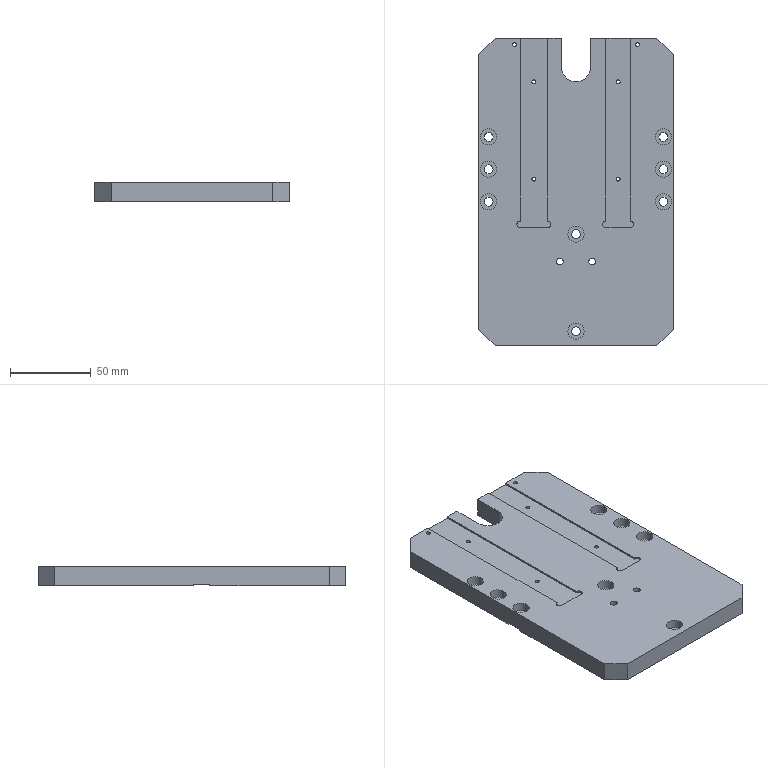Part | STEP file | 2046 Upper blade mounting plate | 1 solid | 88 faces | box 120 x 190 x 12 mm | volume 255418 mm3 | cylinder 55 | plane 33 | commonest cylinder face diameters 5.5 x16 10 x16 2.5 x12 4 x6 4.2 x4 18 x1